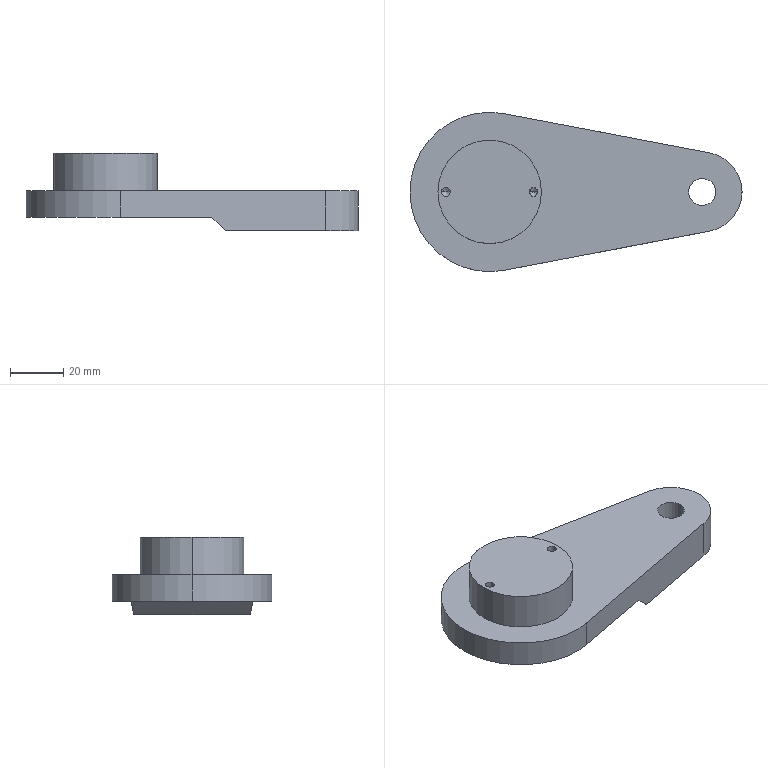Part | STEP file | Driven adjustment support (reverse) QY-1-27 | 1 solid | 22 faces | box 125 x 60 x 29 mm | volume 78443 mm3 | cylinder 11 | plane 7 | cone 4 | commonest cylinder face diameters 3.3 x4 10.2 x2 39 x2 60 x2 30 x1
STEP:
#1=CARTESIAN_POINT('',(0.,0.,0.));
#2=DIRECTION('',(0.,0.,1.));
#3=DIRECTION('',(1.,0.,0.));
#4=AXIS2_PLACEMENT_3D('',#1,#2,#3);
#5=CARTESIAN_POINT('',(-14.85,0.,10.));
#6=VERTEX_POINT('',#5);
#7=CARTESIAN_POINT('',(-14.85,0.,21.5));
#8=VERTEX_POINT('',#7);
#9=CARTESIAN_POINT('',(-14.85,0.,21.5));
#10=DIRECTION('',(0.,0.,1.));
#11=VECTOR('',#10,1.);
#12=LINE('',#9,#11);
#13=CARTESIAN_POINT('',(-16.5,0.,21.5));
#14=DIRECTION('',(0.,0.,1.));
#15=DIRECTION('',(1.,0.,0.));
#16=AXIS2_PLACEMENT_3D('',#13,#14,#15);
#17=CYLINDRICAL_SURFACE('',#16,1.65);
#18=CARTESIAN_POINT('',(6.283,0.));
#19=DIRECTION('',(0.,1.));
#20=VECTOR('',#19,1.);
#21=LINE('',#18,#20);
#22=(GEOMETRIC_REPRESENTATION_CONTEXT(2)PARAMETRIC_REPRESENTATION_CONTEXT()REPRESENTATION_CONTEXT('',''));
#23=DEFINITIONAL_REPRESENTATION('',(#21),#22);
#24=PCURVE('',#17,#23);
#25=CARTESIAN_POINT('',(-16.5,0.,21.5));
#26=DIRECTION('',(0.,0.,1.));
#27=DIRECTION('',(1.,0.,0.));
#28=AXIS2_PLACEMENT_3D('',#25,#26,#27);
#29=CYLINDRICAL_SURFACE('',#28,1.65);
#30=CARTESIAN_POINT('',(0.,0.));
#31=DIRECTION('',(0.,1.));
#32=VECTOR('',#31,1.);
#33=LINE('',#30,#32);
#34=(GEOMETRIC_REPRESENTATION_CONTEXT(2)PARAMETRIC_REPRESENTATION_CONTEXT()REPRESENTATION_CONTEXT('',''));
#35=DEFINITIONAL_REPRESENTATION('',(#33),#34);
#36=PCURVE('',#29,#35);
#37=SURFACE_CURVE('',#12,(#24,#36),.PCURVE_S1.);
#38=EDGE_CURVE('',#6,#8,#37,.T.);
#39=ORIENTED_EDGE('',*,*,#38,.T.);
#40=CARTESIAN_POINT('',(-18.15,0.,21.5));
#41=VERTEX_POINT('',#40);
#42=CARTESIAN_POINT('',(-16.5,0.,21.5));
#43=DIRECTION('',(0.,0.,1.));
#44=DIRECTION('',(1.,0.,0.));
#45=AXIS2_PLACEMENT_3D('',#42,#43,#44);
#46=CIRCLE('',#45,1.65);
#47=CARTESIAN_POINT('',(0.,0.));
#48=DIRECTION('',(1.,0.));
#49=VECTOR('',#48,1.);
#50=LINE('',#47,#49);
#51=(GEOMETRIC_REPRESENTATION_CONTEXT(2)PARAMETRIC_REPRESENTATION_CONTEXT()REPRESENTATION_CONTEXT('',''));
#52=DEFINITIONAL_REPRESENTATION('',(#50),#51);
#53=PCURVE('',#17,#52);
#54=CARTESIAN_POINT('',(0.,0.,21.5));
#55=DIRECTION('',(0.,0.,1.));
#56=DIRECTION('',(1.,0.,0.));
#57=AXIS2_PLACEMENT_3D('',#54,#55,#56);
#58=PLANE('',#57);
#59=CARTESIAN_POINT('',(-16.5,0.));
#60=DIRECTION('',(1.,0.));
#61=AXIS2_PLACEMENT_2D('',#59,#60);
#62=CIRCLE('',#61,1.65);
#63=(GEOMETRIC_REPRESENTATION_CONTEXT(2)PARAMETRIC_REPRESENTATION_CONTEXT()REPRESENTATION_CONTEXT('',''));
#64=DEFINITIONAL_REPRESENTATION('',(#62),#63);
#65=PCURVE('',#58,#64);
#66=SURFACE_CURVE('',#46,(#53,#65),.PCURVE_S1.);
#67=EDGE_CURVE('',#41,#8,#66,.T.);
#68=ORIENTED_EDGE('',*,*,#67,.F.);
#69=CARTESIAN_POINT('',(-18.15,0.,10.));
#70=VERTEX_POINT('',#69);
#71=CARTESIAN_POINT('',(-18.15,0.,21.5));
#72=DIRECTION('',(0.,0.,1.));
#73=VECTOR('',#72,1.);
#74=LINE('',#71,#73);
#75=CARTESIAN_POINT('',(3.142,0.));
#76=DIRECTION('',(0.,1.));
#77=VECTOR('',#76,1.);
#78=LINE('',#75,#77);
#79=(GEOMETRIC_REPRESENTATION_CONTEXT(2)PARAMETRIC_REPRESENTATION_CONTEXT()REPRESENTATION_CONTEXT('',''));
#80=DEFINITIONAL_REPRESENTATION('',(#78),#79);
#81=PCURVE('',#17,#80);
#82=CARTESIAN_POINT('',(3.142,0.));
#83=DIRECTION('',(0.,1.));
#84=VECTOR('',#83,1.);
#85=LINE('',#82,#84);
#86=(GEOMETRIC_REPRESENTATION_CONTEXT(2)PARAMETRIC_REPRESENTATION_CONTEXT()REPRESENTATION_CONTEXT('',''));
#87=DEFINITIONAL_REPRESENTATION('',(#85),#86);
#88=PCURVE('',#29,#87);
#89=SURFACE_CURVE('',#74,(#81,#88),.PCURVE_S1.);
#90=EDGE_CURVE('',#70,#41,#89,.T.);
#91=ORIENTED_EDGE('',*,*,#90,.F.);
#92=CARTESIAN_POINT('',(-16.5,0.,10.));
#93=DIRECTION('',(0.,0.,1.));
#94=DIRECTION('',(1.,0.,0.));
#95=AXIS2_PLACEMENT_3D('',#92,#93,#94);
#96=CIRCLE('',#95,1.65);
#97=CARTESIAN_POINT('',(0.,-11.5));
#98=DIRECTION('',(1.,0.));
#99=VECTOR('',#98,1.);
#100=LINE('',#97,#99);
#101=(GEOMETRIC_REPRESENTATION_CONTEXT(2)PARAMETRIC_REPRESENTATION_CONTEXT()REPRESENTATION_CONTEXT('',''));
#102=DEFINITIONAL_REPRESENTATION('',(#100),#101);
#103=PCURVE('',#17,#102);
#104=CARTESIAN_POINT('',(-16.5,0.,10.));
#105=DIRECTION('',(0.,0.,1.));
#106=DIRECTION('',(1.,0.,0.));
#107=AXIS2_PLACEMENT_3D('',#104,#105,#106);
#108=CONICAL_SURFACE('',#107,1.65,1.03);
#109=CARTESIAN_POINT('',(0.,0.));
#110=DIRECTION('',(1.,0.));
#111=VECTOR('',#110,1.);
#112=LINE('',#109,#111);
#113=(GEOMETRIC_REPRESENTATION_CONTEXT(2)PARAMETRIC_REPRESENTATION_CONTEXT()REPRESENTATION_CONTEXT('',''));
#114=DEFINITIONAL_REPRESENTATION('',(#112),#113);
#115=PCURVE('',#108,#114);
#116=SURFACE_CURVE('',#96,(#103,#115),.PCURVE_S1.);
#117=EDGE_CURVE('',#70,#6,#116,.T.);
#118=ORIENTED_EDGE('',*,*,#117,.T.);
#119=EDGE_LOOP('',(#39,#68,#91,#118));
#120=FACE_BOUND('',#119,.F.);
#121=ADVANCED_FACE('',(#120),#17,.F.);
#122=ORIENTED_EDGE('',*,*,#117,.F.);
#123=CARTESIAN_POINT('',(-16.5,0.,9.009));
#124=VERTEX_POINT('',#123);
#125=CARTESIAN_POINT('',(-18.15,0.,10.));
#126=DIRECTION('',(-0.8572,0.,0.515));
#127=VECTOR('',#126,1.);
#128=LINE('',#125,#127);
#129=CARTESIAN_POINT('',(3.142,0.));
#130=DIRECTION('',(0.,1.));
#131=VECTOR('',#130,1.);
#132=LINE('',#129,#131);
#133=(GEOMETRIC_REPRESENTATION_CONTEXT(2)PARAMETRIC_REPRESENTATION_CONTEXT()REPRESENTATION_CONTEXT('',''));
#134=DEFINITIONAL_REPRESENTATION('',(#132),#133);
#135=PCURVE('',#108,#134);
#136=CARTESIAN_POINT('',(-16.5,0.,10.));
#137=DIRECTION('',(0.,0.,1.));
#138=DIRECTION('',(1.,0.,0.));
#139=AXIS2_PLACEMENT_3D('',#136,#137,#138);
#140=CONICAL_SURFACE('',#139,1.65,1.03);
#141=CARTESIAN_POINT('',(3.142,0.));
#142=DIRECTION('',(0.,1.));
#143=VECTOR('',#142,1.);
#144=LINE('',#141,#143);
#145=(GEOMETRIC_REPRESENTATION_CONTEXT(2)PARAMETRIC_REPRESENTATION_CONTEXT()REPRESENTATION_CONTEXT('',''));
#146=DEFINITIONAL_REPRESENTATION('',(#144),#145);
#147=PCURVE('',#140,#146);
#148=SURFACE_CURVE('',#128,(#135,#147),.PCURVE_S1.);
#149=EDGE_CURVE('',#124,#70,#148,.T.);
#150=ORIENTED_EDGE('',*,*,#149,.F.);
#151=CARTESIAN_POINT('',(-14.85,0.,10.));
#152=DIRECTION('',(0.8572,0.,0.515));
#153=VECTOR('',#152,1.);
#154=LINE('',#151,#153);
#155=CARTESIAN_POINT('',(6.283,0.));
#156=DIRECTION('',(0.,1.));
#157=VECTOR('',#156,1.);
#158=LINE('',#155,#157);
#159=(GEOMETRIC_REPRESENTATION_CONTEXT(2)PARAMETRIC_REPRESENTATION_CONTEXT()REPRESENTATION_CONTEXT('',''));
#160=DEFINITIONAL_REPRESENTATION('',(#158),#159);
#161=PCURVE('',#108,#160);
#162=CARTESIAN_POINT('',(0.,0.));
#163=DIRECTION('',(0.,1.));
#164=VECTOR('',#163,1.);
#165=LINE('',#162,#164);
#166=(GEOMETRIC_REPRESENTATION_CONTEXT(2)PARAMETRIC_REPRESENTATION_CONTEXT()REPRESENTATION_CONTEXT('',''));
#167=DEFINITIONAL_REPRESENTATION('',(#165),#166);
#168=PCURVE('',#140,#167);
#169=SURFACE_CURVE('',#154,(#161,#168),.PCURVE_S1.);
#170=EDGE_CURVE('',#124,#6,#169,.T.);
#171=ORIENTED_EDGE('',*,*,#170,.T.);
#172=EDGE_LOOP('',(#122,#150,#171));
#173=FACE_BOUND('',#172,.F.);
#174=ADVANCED_FACE('',(#173),#108,.F.);
#175=CARTESIAN_POINT('',(18.15,0.,10.));
#176=VERTEX_POINT('',#175);
#177=CARTESIAN_POINT('',(18.15,0.,21.5));
#178=VERTEX_POINT('',#177);
#179=CARTESIAN_POINT('',(18.15,0.,21.5));
#180=DIRECTION('',(0.,0.,1.));
#181=VECTOR('',#180,1.);
#182=LINE('',#179,#181);
#183=CARTESIAN_POINT('',(16.5,0.,21.5));
#184=DIRECTION('',(0.,0.,1.));
#185=DIRECTION('',(1.,0.,0.));
#186=AXIS2_PLACEMENT_3D('',#183,#184,#185);
#187=CYLINDRICAL_SURFACE('',#186,1.65);
#188=CARTESIAN_POINT('',(6.283,0.));
#189=DIRECTION('',(0.,1.));
#190=VECTOR('',#189,1.);
#191=LINE('',#188,#190);
#192=(GEOMETRIC_REPRESENTATION_CONTEXT(2)PARAMETRIC_REPRESENTATION_CONTEXT()REPRESENTATION_CONTEXT('',''));
#193=DEFINITIONAL_REPRESENTATION('',(#191),#192);
#194=PCURVE('',#187,#193);
#195=CARTESIAN_POINT('',(16.5,0.,21.5));
#196=DIRECTION('',(0.,0.,1.));
#197=DIRECTION('',(1.,0.,0.));
#198=AXIS2_PLACEMENT_3D('',#195,#196,#197);
#199=CYLINDRICAL_SURFACE('',#198,1.65);
#200=CARTESIAN_POINT('',(0.,0.));
#201=DIRECTION('',(0.,1.));
#202=VECTOR('',#201,1.);
#203=LINE('',#200,#202);
#204=(GEOMETRIC_REPRESENTATION_CONTEXT(2)PARAMETRIC_REPRESENTATION_CONTEXT()REPRESENTATION_CONTEXT('',''));
#205=DEFINITIONAL_REPRESENTATION('',(#203),#204);
#206=PCURVE('',#199,#205);
#207=SURFACE_CURVE('',#182,(#194,#206),.PCURVE_S1.);
#208=EDGE_CURVE('',#176,#178,#207,.T.);
#209=ORIENTED_EDGE('',*,*,#208,.T.);
#210=CARTESIAN_POINT('',(14.85,0.,21.5));
#211=VERTEX_POINT('',#210);
#212=CARTESIAN_POINT('',(16.5,0.,21.5));
#213=DIRECTION('',(0.,0.,1.));
#214=DIRECTION('',(1.,0.,0.));
#215=AXIS2_PLACEMENT_3D('',#212,#213,#214);
#216=CIRCLE('',#215,1.65);
#217=CARTESIAN_POINT('',(0.,0.));
#218=DIRECTION('',(1.,0.));
#219=VECTOR('',#218,1.);
#220=LINE('',#217,#219);
#221=(GEOMETRIC_REPRESENTATION_CONTEXT(2)PARAMETRIC_REPRESENTATION_CONTEXT()REPRESENTATION_CONTEXT('',''));
#222=DEFINITIONAL_REPRESENTATION('',(#220),#221);
#223=PCURVE('',#187,#222);
#224=CARTESIAN_POINT('',(16.5,0.));
#225=DIRECTION('',(1.,0.));
#226=AXIS2_PLACEMENT_2D('',#224,#225);
#227=CIRCLE('',#226,1.65);
#228=(GEOMETRIC_REPRESENTATION_CONTEXT(2)PARAMETRIC_REPRESENTATION_CONTEXT()REPRESENTATION_CONTEXT('',''));
#229=DEFINITIONAL_REPRESENTATION('',(#227),#228);
#230=PCURVE('',#58,#229);
#231=SURFACE_CURVE('',#216,(#223,#230),.PCURVE_S1.);
#232=EDGE_CURVE('',#211,#178,#231,.T.);
#233=ORIENTED_EDGE('',*,*,#232,.F.);
#234=CARTESIAN_POINT('',(14.85,0.,10.));
#235=VERTEX_POINT('',#234);
#236=CARTESIAN_POINT('',(14.85,0.,21.5));
#237=DIRECTION('',(0.,0.,1.));
#238=VECTOR('',#237,1.);
#239=LINE('',#236,#238);
#240=CARTESIAN_POINT('',(3.142,0.));
#241=DIRECTION('',(0.,1.));
#242=VECTOR('',#241,1.);
#243=LINE('',#240,#242);
#244=(GEOMETRIC_REPRESENTATION_CONTEXT(2)PARAMETRIC_REPRESENTATION_CONTEXT()REPRESENTATION_CONTEXT('',''));
#245=DEFINITIONAL_REPRESENTATION('',(#243),#244);
#246=PCURVE('',#187,#245);
#247=CARTESIAN_POINT('',(3.142,0.));
#248=DIRECTION('',(0.,1.));
#249=VECTOR('',#248,1.);
#250=LINE('',#247,#249);
#251=(GEOMETRIC_REPRESENTATION_CONTEXT(2)PARAMETRIC_REPRESENTATION_CONTEXT()REPRESENTATION_CONTEXT('',''));
#252=DEFINITIONAL_REPRESENTATION('',(#250),#251);
#253=PCURVE('',#199,#252);
#254=SURFACE_CURVE('',#239,(#246,#253),.PCURVE_S1.);
#255=EDGE_CURVE('',#235,#211,#254,.T.);
#256=ORIENTED_EDGE('',*,*,#255,.F.);
#257=CARTESIAN_POINT('',(16.5,0.,10.));
#258=DIRECTION('',(0.,0.,1.));
#259=DIRECTION('',(1.,0.,0.));
#260=AXIS2_PLACEMENT_3D('',#257,#258,#259);
#261=CIRCLE('',#260,1.65);
#262=CARTESIAN_POINT('',(0.,-11.5));
#263=DIRECTION('',(1.,0.));
#264=VECTOR('',#263,1.);
#265=LINE('',#262,#264);
#266=(GEOMETRIC_REPRESENTATION_CONTEXT(2)PARAMETRIC_REPRESENTATION_CONTEXT()REPRESENTATION_CONTEXT('',''));
#267=DEFINITIONAL_REPRESENTATION('',(#265),#266);
#268=PCURVE('',#187,#267);
#269=CARTESIAN_POINT('',(16.5,0.,10.));
#270=DIRECTION('',(0.,0.,1.));
#271=DIRECTION('',(1.,0.,0.));
#272=AXIS2_PLACEMENT_3D('',#269,#270,#271);
#273=CONICAL_SURFACE('',#272,1.65,1.03);
#274=CARTESIAN_POINT('',(0.,0.));
#275=DIRECTION('',(1.,0.));
#276=VECTOR('',#275,1.);
#277=LINE('',#274,#276);
#278=(GEOMETRIC_REPRESENTATION_CONTEXT(2)PARAMETRIC_REPRESENTATION_CONTEXT()REPRESENTATION_CONTEXT('',''));
#279=DEFINITIONAL_REPRESENTATION('',(#277),#278);
#280=PCURVE('',#273,#279);
#281=SURFACE_CURVE('',#261,(#268,#280),.PCURVE_S1.);
#282=EDGE_CURVE('',#235,#176,#281,.T.);
#283=ORIENTED_EDGE('',*,*,#282,.T.);
#284=EDGE_LOOP('',(#209,#233,#256,#283));
#285=FACE_BOUND('',#284,.F.);
#286=ADVANCED_FACE('',(#285),#187,.F.);
#287=ORIENTED_EDGE('',*,*,#282,.F.);
#288=CARTESIAN_POINT('',(16.5,0.,9.009));
#289=VERTEX_POINT('',#288);
#290=CARTESIAN_POINT('',(14.85,0.,10.));
#291=DIRECTION('',(-0.8572,0.,0.515));
#292=VECTOR('',#291,1.);
#293=LINE('',#290,#292);
#294=CARTESIAN_POINT('',(3.142,0.));
#295=DIRECTION('',(0.,1.));
#296=VECTOR('',#295,1.);
#297=LINE('',#294,#296);
#298=(GEOMETRIC_REPRESENTATION_CONTEXT(2)PARAMETRIC_REPRESENTATION_CONTEXT()REPRESENTATION_CONTEXT('',''));
#299=DEFINITIONAL_REPRESENTATION('',(#297),#298);
#300=PCURVE('',#273,#299);
#301=CARTESIAN_POINT('',(16.5,0.,10.));
#302=DIRECTION('',(0.,0.,1.));
#303=DIRECTION('',(1.,0.,0.));
#304=AXIS2_PLACEMENT_3D('',#301,#302,#303);
#305=CONICAL_SURFACE('',#304,1.65,1.03);
#306=CARTESIAN_POINT('',(3.142,0.));
#307=DIRECTION('',(0.,1.));
#308=VECTOR('',#307,1.);
#309=LINE('',#306,#308);
#310=(GEOMETRIC_REPRESENTATION_CONTEXT(2)PARAMETRIC_REPRESENTATION_CONTEXT()REPRESENTATION_CONTEXT('',''));
#311=DEFINITIONAL_REPRESENTATION('',(#309),#310);
#312=PCURVE('',#305,#311);
#313=SURFACE_CURVE('',#293,(#300,#312),.PCURVE_S1.);
#314=EDGE_CURVE('',#289,#235,#313,.T.);
#315=ORIENTED_EDGE('',*,*,#314,.F.);
#316=CARTESIAN_POINT('',(18.15,0.,10.));
#317=DIRECTION('',(0.8572,0.,0.515));
#318=VECTOR('',#317,1.);
#319=LINE('',#316,#318);
#320=CARTESIAN_POINT('',(6.283,0.));
#321=DIRECTION('',(0.,1.));
#322=VECTOR('',#321,1.);
#323=LINE('',#320,#322);
#324=(GEOMETRIC_REPRESENTATION_CONTEXT(2)PARAMETRIC_REPRESENTATION_CONTEXT()REPRESENTATION_CONTEXT('',''));
#325=DEFINITIONAL_REPRESENTATION('',(#323),#324);
#326=PCURVE('',#273,#325);
#327=CARTESIAN_POINT('',(0.,0.));
#328=DIRECTION('',(0.,1.));
#329=VECTOR('',#328,1.);
#330=LINE('',#327,#329);
#331=(GEOMETRIC_REPRESENTATION_CONTEXT(2)PARAMETRIC_REPRESENTATION_CONTEXT()REPRESENTATION_CONTEXT('',''));
#332=DEFINITIONAL_REPRESENTATION('',(#330),#331);
#333=PCURVE('',#305,#332);
#334=SURFACE_CURVE('',#319,(#326,#333),.PCURVE_S1.);
#335=EDGE_CURVE('',#289,#176,#334,.T.);
#336=ORIENTED_EDGE('',*,*,#335,.T.);
#337=EDGE_LOOP('',(#287,#315,#336));
#338=FACE_BOUND('',#337,.F.);
#339=ADVANCED_FACE('',(#338),#273,.F.);
#340=CARTESIAN_POINT('',(19.5,0.,21.5));
#341=VERTEX_POINT('',#340);
#342=CARTESIAN_POINT('',(-19.5,0.,21.5));
#343=VERTEX_POINT('',#342);
#344=CARTESIAN_POINT('',(0.,0.,21.5));
#345=DIRECTION('',(0.,0.,1.));
#346=DIRECTION('',(1.,0.,0.));
#347=AXIS2_PLACEMENT_3D('',#344,#345,#346);
#348=CIRCLE('',#347,19.5);
#349=CARTESIAN_POINT('',(0.,0.,21.5));
#350=DIRECTION('',(0.,0.,-1.));
#351=DIRECTION('',(-1.,0.,0.));
#352=AXIS2_PLACEMENT_3D('',#349,#350,#351);
#353=CYLINDRICAL_SURFACE('',#352,19.5);
#354=CARTESIAN_POINT('',(3.142,0.));
#355=DIRECTION('',(-1.,0.));
#356=VECTOR('',#355,1.);
#357=LINE('',#354,#356);
#358=(GEOMETRIC_REPRESENTATION_CONTEXT(2)PARAMETRIC_REPRESENTATION_CONTEXT()REPRESENTATION_CONTEXT('',''));
#359=DEFINITIONAL_REPRESENTATION('',(#357),#358);
#360=PCURVE('',#353,#359);
#361=CARTESIAN_POINT('',(0.,0.));
#362=DIRECTION('',(1.,0.));
#363=AXIS2_PLACEMENT_2D('',#361,#362);
#364=CIRCLE('',#363,19.5);
#365=(GEOMETRIC_REPRESENTATION_CONTEXT(2)PARAMETRIC_REPRESENTATION_CONTEXT()REPRESENTATION_CONTEXT('',''));
#366=DEFINITIONAL_REPRESENTATION('',(#364),#365);
#367=PCURVE('',#58,#366);
#368=SURFACE_CURVE('',#348,(#360,#367),.PCURVE_S1.);
#369=EDGE_CURVE('',#341,#343,#368,.T.);
#370=ORIENTED_EDGE('',*,*,#369,.F.);
#371=CARTESIAN_POINT('',(19.5,0.,7.5));
#372=VERTEX_POINT('',#371);
#373=CARTESIAN_POINT('',(19.5,0.,21.5));
#374=DIRECTION('',(0.,0.,-1.));
#375=VECTOR('',#374,1.);
#376=LINE('',#373,#375);
#377=CARTESIAN_POINT('',(3.142,0.));
#378=DIRECTION('',(0.,1.));
#379=VECTOR('',#378,1.);
#380=LINE('',#377,#379);
#381=(GEOMETRIC_REPRESENTATION_CONTEXT(2)PARAMETRIC_REPRESENTATION_CONTEXT()REPRESENTATION_CONTEXT('',''));
#382=DEFINITIONAL_REPRESENTATION('',(#380),#381);
#383=PCURVE('',#353,#382);
#384=CARTESIAN_POINT('',(0.,0.,21.5));
#385=DIRECTION('',(0.,0.,-1.));
#386=DIRECTION('',(-1.,0.,0.));
#387=AXIS2_PLACEMENT_3D('',#384,#385,#386);
#388=CYLINDRICAL_SURFACE('',#387,19.5);
#389=CARTESIAN_POINT('',(3.142,0.));
#390=DIRECTION('',(0.,1.));
#391=VECTOR('',#390,1.);
#392=LINE('',#389,#391);
#393=(GEOMETRIC_REPRESENTATION_CONTEXT(2)PARAMETRIC_REPRESENTATION_CONTEXT()REPRESENTATION_CONTEXT('',''));
#394=DEFINITIONAL_REPRESENTATION('',(#392),#393);
#395=PCURVE('',#388,#394);
#396=SURFACE_CURVE('',#376,(#383,#395),.PCURVE_S1.);
#397=EDGE_CURVE('',#341,#372,#396,.T.);
#398=ORIENTED_EDGE('',*,*,#397,.T.);
#399=CARTESIAN_POINT('',(-19.5,0.,7.5));
#400=VERTEX_POINT('',#399);
#401=CARTESIAN_POINT('',(0.,0.,7.5));
#402=DIRECTION('',(0.,0.,1.));
#403=DIRECTION('',(1.,0.,0.));
#404=AXIS2_PLACEMENT_3D('',#401,#402,#403);
#405=CIRCLE('',#404,19.5);
#406=CARTESIAN_POINT('',(3.142,14.));
#407=DIRECTION('',(-1.,0.));
#408=VECTOR('',#407,1.);
#409=LINE('',#406,#408);
#410=(GEOMETRIC_REPRESENTATION_CONTEXT(2)PARAMETRIC_REPRESENTATION_CONTEXT()REPRESENTATION_CONTEXT('',''));
#411=DEFINITIONAL_REPRESENTATION('',(#409),#410);
#412=PCURVE('',#353,#411);
#413=CARTESIAN_POINT('',(0.,0.,7.5));
#414=DIRECTION('',(0.,0.,1.));
#415=DIRECTION('',(1.,0.,0.));
#416=AXIS2_PLACEMENT_3D('',#413,#414,#415);
#417=PLANE('',#416);
#418=CARTESIAN_POINT('',(0.,0.));
#419=DIRECTION('',(1.,0.));
#420=AXIS2_PLACEMENT_2D('',#418,#419);
#421=CIRCLE('',#420,19.5);
#422=(GEOMETRIC_REPRESENTATION_CONTEXT(2)PARAMETRIC_REPRESENTATION_CONTEXT()REPRESENTATION_CONTEXT('',''));
#423=DEFINITIONAL_REPRESENTATION('',(#421),#422);
#424=PCURVE('',#417,#423);
#425=SURFACE_CURVE('',#405,(#412,#424),.PCURVE_S1.);
#426=EDGE_CURVE('',#372,#400,#425,.T.);
#427=ORIENTED_EDGE('',*,*,#426,.T.);
#428=CARTESIAN_POINT('',(-19.5,0.,21.5));
#429=DIRECTION('',(0.,0.,-1.));
#430=VECTOR('',#429,1.);
#431=LINE('',#428,#430);
#432=CARTESIAN_POINT('',(0.,0.));
#433=DIRECTION('',(0.,1.));
#434=VECTOR('',#433,1.);
#435=LINE('',#432,#434);
#436=(GEOMETRIC_REPRESENTATION_CONTEXT(2)PARAMETRIC_REPRESENTATION_CONTEXT()REPRESENTATION_CONTEXT('',''));
#437=DEFINITIONAL_REPRESENTATION('',(#435),#436);
#438=PCURVE('',#353,#437);
#439=CARTESIAN_POINT('',(6.283,0.));
#440=DIRECTION('',(0.,1.));
#441=VECTOR('',#440,1.);
#442=LINE('',#439,#441);
#443=(GEOMETRIC_REPRESENTATION_CONTEXT(2)PARAMETRIC_REPRESENTATION_CONTEXT()REPRESENTATION_CONTEXT('',''));
#444=DEFINITIONAL_REPRESENTATION('',(#442),#443);
#445=PCURVE('',#388,#444);
#446=SURFACE_CURVE('',#431,(#438,#445),.PCURVE_S1.);
#447=EDGE_CURVE('',#343,#400,#446,.T.);
#448=ORIENTED_EDGE('',*,*,#447,.F.);
#449=EDGE_LOOP('',(#370,#398,#427,#448));
#450=FACE_BOUND('',#449,.T.);
#451=ADVANCED_FACE('',(#450),#353,.T.);
#452=CARTESIAN_POINT('',(74.9,0.,7.5));
#453=VERTEX_POINT('',#452);
#454=CARTESIAN_POINT('',(74.9,0.,-7.5));
#455=VERTEX_POINT('',#454);
#456=CARTESIAN_POINT('',(74.9,0.,-7.5));
#457=DIRECTION('',(0.,0.,-1.));
#458=VECTOR('',#457,1.);
#459=LINE('',#456,#458);
#460=CARTESIAN_POINT('',(80.,0.,-7.5));
#461=DIRECTION('',(0.,0.,-1.));
#462=DIRECTION('',(-1.,0.,0.));
#463=AXIS2_PLACEMENT_3D('',#460,#461,#462);
#464=CYLINDRICAL_SURFACE('',#463,5.1);
#465=CARTESIAN_POINT('',(6.283,0.));
#466=DIRECTION('',(0.,1.));
#467=VECTOR('',#466,1.);
#468=LINE('',#465,#467);
#469=(GEOMETRIC_REPRESENTATION_CONTEXT(2)PARAMETRIC_REPRESENTATION_CONTEXT()REPRESENTATION_CONTEXT('',''));
#470=DEFINITIONAL_REPRESENTATION('',(#468),#469);
#471=PCURVE('',#464,#470);
#472=CARTESIAN_POINT('',(80.,0.,-7.5));
#473=DIRECTION('',(0.,0.,-1.));
#474=DIRECTION('',(-1.,0.,0.));
#475=AXIS2_PLACEMENT_3D('',#472,#473,#474);
#476=CYLINDRICAL_SURFACE('',#475,5.1);
#477=CARTESIAN_POINT('',(0.,0.));
#478=DIRECTION('',(0.,1.));
#479=VECTOR('',#478,1.);
#480=LINE('',#477,#479);
#481=(GEOMETRIC_REPRESENTATION_CONTEXT(2)PARAMETRIC_REPRESENTATION_CONTEXT()REPRESENTATION_CONTEXT('',''));
#482=DEFINITIONAL_REPRESENTATION('',(#480),#481);
#483=PCURVE('',#476,#482);
#484=SURFACE_CURVE('',#459,(#471,#483),.PCURVE_S1.);
#485=EDGE_CURVE('',#453,#455,#484,.T.);
#486=ORIENTED_EDGE('',*,*,#485,.T.);
#487=CARTESIAN_POINT('',(85.1,0.,-7.5));
#488=VERTEX_POINT('',#487);
#489=CARTESIAN_POINT('',(80.,0.,-7.5));
#490=DIRECTION('',(0.,0.,-1.));
#491=DIRECTION('',(-1.,0.,0.));
#492=AXIS2_PLACEMENT_3D('',#489,#490,#491);
#493=CIRCLE('',#492,5.1);
#494=CARTESIAN_POINT('',(0.,0.));
#495=DIRECTION('',(1.,0.));
#496=VECTOR('',#495,1.);
#497=LINE('',#494,#496);
#498=(GEOMETRIC_REPRESENTATION_CONTEXT(2)PARAMETRIC_REPRESENTATION_CONTEXT()REPRESENTATION_CONTEXT('',''));
#499=DEFINITIONAL_REPRESENTATION('',(#497),#498);
#500=PCURVE('',#464,#499);
#501=CARTESIAN_POINT('',(0.,0.,-7.5));
#502=DIRECTION('',(0.,0.,1.));
#503=DIRECTION('',(1.,0.,0.));
#504=AXIS2_PLACEMENT_3D('',#501,#502,#503);
#505=PLANE('',#504);
#506=CARTESIAN_POINT('',(74.9,0.));
#507=CARTESIAN_POINT('',(74.9,8.833));
#508=CARTESIAN_POINT('',(82.55,4.417));
#509=CARTESIAN_POINT('',(90.2,0.));
#510=CARTESIAN_POINT('',(82.55,-4.417));
#511=CARTESIAN_POINT('',(74.9,-8.833));
#512=CARTESIAN_POINT('',(74.9,0.));
#513=(BOUNDED_CURVE()B_SPLINE_CURVE(2,(#506,#507,#508,#509,#510,#511,#512),.UNSPECIFIED.,.T.,.F.)B_SPLINE_CURVE_WITH_KNOTS((1,2,2,2,2,1),(-2.094,0.,2.094,4.189,6.283,8.378),.UNSPECIFIED.)CURVE()GEOMETRIC_REPRESENTATION_ITEM()RATIONAL_B_SPLINE_CURVE((1.,0.5,1.,0.5,1.,0.5,1.))REPRESENTATION_ITEM(''));
#514=(GEOMETRIC_REPRESENTATION_CONTEXT(2)PARAMETRIC_REPRESENTATION_CONTEXT()REPRESENTATION_CONTEXT('',''));
#515=DEFINITIONAL_REPRESENTATION('',(#513),#514);
#516=PCURVE('',#505,#515);
#517=SURFACE_CURVE('',#493,(#500,#516),.PCURVE_S1.);
#518=EDGE_CURVE('',#488,#455,#517,.T.);
#519=ORIENTED_EDGE('',*,*,#518,.F.);
#520=CARTESIAN_POINT('',(85.1,0.,7.5));
#521=VERTEX_POINT('',#520);
#522=CARTESIAN_POINT('',(85.1,0.,-7.5));
#523=DIRECTION('',(0.,0.,-1.));
#524=VECTOR('',#523,1.);
#525=LINE('',#522,#524);
#526=CARTESIAN_POINT('',(3.142,0.));
#527=DIRECTION('',(0.,1.));
#528=VECTOR('',#527,1.);
#529=LINE('',#526,#528);
#530=(GEOMETRIC_REPRESENTATION_CONTEXT(2)PARAMETRIC_REPRESENTATION_CONTEXT()REPRESENTATION_CONTEXT('',''));
#531=DEFINITIONAL_REPRESENTATION('',(#529),#530);
#532=PCURVE('',#464,#531);
#533=CARTESIAN_POINT('',(3.142,0.));
#534=DIRECTION('',(0.,1.));
#535=VECTOR('',#534,1.);
#536=LINE('',#533,#535);
#537=(GEOMETRIC_REPRESENTATION_CONTEXT(2)PARAMETRIC_REPRESENTATION_CONTEXT()REPRESENTATION_CONTEXT('',''));
#538=DEFINITIONAL_REPRESENTATION('',(#536),#537);
#539=PCURVE('',#476,#538);
#540=SURFACE_CURVE('',#525,(#532,#539),.PCURVE_S1.);
#541=EDGE_CURVE('',#521,#488,#540,.T.);
#542=ORIENTED_EDGE('',*,*,#541,.F.);
#543=CARTESIAN_POINT('',(80.,0.,7.5));
#544=DIRECTION('',(0.,0.,1.));
#545=DIRECTION('',(1.,0.,0.));
#546=AXIS2_PLACEMENT_3D('',#543,#544,#545);
#547=CIRCLE('',#546,5.1);
#548=CARTESIAN_POINT('',(9.425,-15.));
#549=DIRECTION('',(-1.,0.));
#550=VECTOR('',#549,1.);
#551=LINE('',#548,#550);
#552=(GEOMETRIC_REPRESENTATION_CONTEXT(2)PARAMETRIC_REPRESENTATION_CONTEXT()REPRESENTATION_CONTEXT('',''));
#553=DEFINITIONAL_REPRESENTATION('',(#551),#552);
#554=PCURVE('',#464,#553);
#555=CARTESIAN_POINT('',(80.,0.));
#556=DIRECTION('',(1.,0.));
#557=AXIS2_PLACEMENT_2D('',#555,#556);
#558=CIRCLE('',#557,5.1);
#559=(GEOMETRIC_REPRESENTATION_CONTEXT(2)PARAMETRIC_REPRESENTATION_CONTEXT()REPRESENTATION_CONTEXT('',''));
#560=DEFINITIONAL_REPRESENTATION('',(#558),#559);
#561=PCURVE('',#417,#560);
#562=SURFACE_CURVE('',#547,(#554,#561),.PCURVE_S1.);
#563=EDGE_CURVE('',#453,#521,#562,.T.);
#564=ORIENTED_EDGE('',*,*,#563,.F.);
#565=EDGE_LOOP('',(#486,#519,#542,#564));
#566=FACE_BOUND('',#565,.F.);
#567=ADVANCED_FACE('',(#566),#464,.F.);
#568=CARTESIAN_POINT('',(-30.,0.,7.5));
#569=VERTEX_POINT('',#568);
#570=CARTESIAN_POINT('',(5.625,-29.468,7.5));
#571=VERTEX_POINT('',#570);
#572=CARTESIAN_POINT('',(0.,0.,7.5));
#573=DIRECTION('',(0.,0.,1.));
#574=DIRECTION('',(1.,0.,0.));
#575=AXIS2_PLACEMENT_3D('',#572,#573,#574);
#576=CIRCLE('',#575,30.);
#577=CARTESIAN_POINT('',(0.,0.,7.5));
#578=DIRECTION('',(0.,0.,-1.));
#579=DIRECTION('',(-1.,0.,0.));
#580=AXIS2_PLACEMENT_3D('',#577,#578,#579);
#581=CYLINDRICAL_SURFACE('',#580,30.);
#582=CARTESIAN_POINT('',(9.425,0.));
#583=DIRECTION('',(-1.,0.));
#584=VECTOR('',#583,1.);
#585=LINE('',#582,#584);
#586=(GEOMETRIC_REPRESENTATION_CONTEXT(2)PARAMETRIC_REPRESENTATION_CONTEXT()REPRESENTATION_CONTEXT('',''));
#587=DEFINITIONAL_REPRESENTATION('',(#585),#586);
#588=PCURVE('',#581,#587);
#589=CARTESIAN_POINT('',(0.,0.));
#590=DIRECTION('',(1.,0.));
#591=AXIS2_PLACEMENT_2D('',#589,#590);
#592=CIRCLE('',#591,30.);
#593=(GEOMETRIC_REPRESENTATION_CONTEXT(2)PARAMETRIC_REPRESENTATION_CONTEXT()REPRESENTATION_CONTEXT('',''));
#594=DEFINITIONAL_REPRESENTATION('',(#592),#593);
#595=PCURVE('',#417,#594);
#596=SURFACE_CURVE('',#576,(#588,#595),.PCURVE_S1.);
#597=EDGE_CURVE('',#569,#571,#596,.T.);
#598=ORIENTED_EDGE('',*,*,#597,.F.);
#599=CARTESIAN_POINT('',(-30.,0.,-2.5));
#600=VERTEX_POINT('',#599);
#601=CARTESIAN_POINT('',(-30.,0.,7.5));
#602=DIRECTION('',(0.,0.,-1.));
#603=VECTOR('',#602,1.);
#604=LINE('',#601,#603);
#605=CARTESIAN_POINT('',(6.283,0.));
#606=DIRECTION('',(0.,1.));
#607=VECTOR('',#606,1.);
#608=LINE('',#605,#607);
#609=(GEOMETRIC_REPRESENTATION_CONTEXT(2)PARAMETRIC_REPRESENTATION_CONTEXT()REPRESENTATION_CONTEXT('',''));
#610=DEFINITIONAL_REPRESENTATION('',(#608),#609);
#611=PCURVE('',#581,#610);
#612=CARTESIAN_POINT('',(0.,0.,7.5));
#613=DIRECTION('',(0.,0.,-1.));
#614=DIRECTION('',(-1.,0.,0.));
#615=AXIS2_PLACEMENT_3D('',#612,#613,#614);
#616=CYLINDRICAL_SURFACE('',#615,30.);
#617=CARTESIAN_POINT('',(0.,0.));
#618=DIRECTION('',(0.,1.));
#619=VECTOR('',#618,1.);
#620=LINE('',#617,#619);
#621=(GEOMETRIC_REPRESENTATION_CONTEXT(2)PARAMETRIC_REPRESENTATION_CONTEXT()REPRESENTATION_CONTEXT('',''));
#622=DEFINITIONAL_REPRESENTATION('',(#620),#621);
#623=PCURVE('',#616,#622);
#624=SURFACE_CURVE('',#604,(#611,#623),.PCURVE_S1.);
#625=EDGE_CURVE('',#569,#600,#624,.T.);
#626=ORIENTED_EDGE('',*,*,#625,.T.);
#627=CARTESIAN_POINT('',(5.625,-29.468,-2.5));
#628=VERTEX_POINT('',#627);
#629=CARTESIAN_POINT('',(0.,0.,-2.5));
#630=DIRECTION('',(0.,0.,1.));
#631=DIRECTION('',(1.,0.,0.));
#632=AXIS2_PLACEMENT_3D('',#629,#630,#631);
#633=CIRCLE('',#632,30.);
#634=CARTESIAN_POINT('',(9.425,10.));
#635=DIRECTION('',(-1.,0.));
#636=VECTOR('',#635,1.);
#637=LINE('',#634,#636);
#638=(GEOMETRIC_REPRESENTATION_CONTEXT(2)PARAMETRIC_REPRESENTATION_CONTEXT()REPRESENTATION_CONTEXT('',''));
#639=DEFINITIONAL_REPRESENTATION('',(#637),#638);
#640=PCURVE('',#581,#639);
#641=CARTESIAN_POINT('',(-30.,-50.,-2.5));
#642=DIRECTION('',(0.,0.,1.));
#643=DIRECTION('',(1.,0.,0.));
#644=AXIS2_PLACEMENT_3D('',#641,#642,#643);
#645=PLANE('',#644);
#646=CARTESIAN_POINT('',(30.,50.));
#647=DIRECTION('',(1.,0.));
#648=AXIS2_PLACEMENT_2D('',#646,#647);
#649=CIRCLE('',#648,30.);
#650=(GEOMETRIC_REPRESENTATION_CONTEXT(2)PARAMETRIC_REPRESENTATION_CONTEXT()REPRESENTATION_CONTEXT('',''));
#651=DEFINITIONAL_REPRESENTATION('',(#649),#650);
#652=PCURVE('',#645,#651);
#653=SURFACE_CURVE('',#633,(#640,#652),.PCURVE_S1.);
#654=EDGE_CURVE('',#600,#628,#653,.T.);
#655=ORIENTED_EDGE('',*,*,#654,.T.);
#656=CARTESIAN_POINT('',(5.625,-29.468,7.5));
#657=DIRECTION('',(0.,0.,-1.));
#658=VECTOR('',#657,1.);
#659=LINE('',#656,#658);
#660=CARTESIAN_POINT('',(4.524,0.));
#661=DIRECTION('',(0.,1.));
#662=VECTOR('',#661,1.);
#663=LINE('',#660,#662);
#664=(GEOMETRIC_REPRESENTATION_CONTEXT(2)PARAMETRIC_REPRESENTATION_CONTEXT()REPRESENTATION_CONTEXT('',''));
#665=DEFINITIONAL_REPRESENTATION('',(#663),#664);
#666=PCURVE('',#581,#665);
#667=CARTESIAN_POINT('',(5.625,-29.468,7.5));
#668=DIRECTION('',(-0.1875,0.9823,0.));
#669=DIRECTION('',(-0.9823,-0.1875,0.));
#670=AXIS2_PLACEMENT_3D('',#667,#668,#669);
#671=PLANE('',#670);
#672=CARTESIAN_POINT('',(0.,0.));
#673=DIRECTION('',(0.,-1.));
#674=VECTOR('',#673,1.);
#675=LINE('',#672,#674);
#676=(GEOMETRIC_REPRESENTATION_CONTEXT(2)PARAMETRIC_REPRESENTATION_CONTEXT()REPRESENTATION_CONTEXT('',''));
#677=DEFINITIONAL_REPRESENTATION('',(#675),#676);
#678=PCURVE('',#671,#677);
#679=SURFACE_CURVE('',#659,(#666,#678),.PCURVE_S1.);
#680=EDGE_CURVE('',#571,#628,#679,.T.);
#681=ORIENTED_EDGE('',*,*,#680,.F.);
#682=EDGE_LOOP('',(#598,#626,#655,#681));
#683=FACE_BOUND('',#682,.T.);
#684=ADVANCED_FACE('',(#683),#581,.T.);
#685=ORIENTED_EDGE('',*,*,#625,.F.);
#686=CARTESIAN_POINT('',(5.625,29.468,7.5));
#687=VERTEX_POINT('',#686);
#688=CARTESIAN_POINT('',(0.,0.,7.5));
#689=DIRECTION('',(0.,0.,1.));
#690=DIRECTION('',(1.,0.,0.));
#691=AXIS2_PLACEMENT_3D('',#688,#689,#690);
#692=CIRCLE('',#691,30.);
#693=CARTESIAN_POINT('',(3.142,0.));
#694=DIRECTION('',(-1.,0.));
#695=VECTOR('',#694,1.);
#696=LINE('',#693,#695);
#697=(GEOMETRIC_REPRESENTATION_CONTEXT(2)PARAMETRIC_REPRESENTATION_CONTEXT()REPRESENTATION_CONTEXT('',''));
#698=DEFINITIONAL_REPRESENTATION('',(#696),#697);
#699=PCURVE('',#616,#698);
#700=CARTESIAN_POINT('',(0.,0.));
#701=DIRECTION('',(1.,0.));
#702=AXIS2_PLACEMENT_2D('',#700,#701);
#703=CIRCLE('',#702,30.);
#704=(GEOMETRIC_REPRESENTATION_CONTEXT(2)PARAMETRIC_REPRESENTATION_CONTEXT()REPRESENTATION_CONTEXT('',''));
#705=DEFINITIONAL_REPRESENTATION('',(#703),#704);
#706=PCURVE('',#417,#705);
#707=SURFACE_CURVE('',#692,(#699,#706),.PCURVE_S1.);
#708=EDGE_CURVE('',#687,#569,#707,.T.);
#709=ORIENTED_EDGE('',*,*,#708,.F.);
#710=CARTESIAN_POINT('',(5.625,29.468,-2.5));
#711=VERTEX_POINT('',#710);
#712=CARTESIAN_POINT('',(5.625,29.468,7.5));
#713=DIRECTION('',(0.,0.,-1.));
#714=VECTOR('',#713,1.);
#715=LINE('',#712,#714);
#716=CARTESIAN_POINT('',(1.759,0.));
#717=DIRECTION('',(0.,1.));
#718=VECTOR('',#717,1.);
#719=LINE('',#716,#718);
#720=(GEOMETRIC_REPRESENTATION_CONTEXT(2)PARAMETRIC_REPRESENTATION_CONTEXT()REPRESENTATION_CONTEXT('',''));
#721=DEFINITIONAL_REPRESENTATION('',(#719),#720);
#722=PCURVE('',#616,#721);
#723=CARTESIAN_POINT('',(5.625,29.468,7.5));
#724=DIRECTION('',(-0.1875,-0.9823,0.));
#725=DIRECTION('',(0.9823,-0.1875,0.));
#726=AXIS2_PLACEMENT_3D('',#723,#724,#725);
#727=PLANE('',#726);
#728=CARTESIAN_POINT('',(0.,0.));
#729=DIRECTION('',(0.,-1.));
#730=VECTOR('',#729,1.);
#731=LINE('',#728,#730);
#732=(GEOMETRIC_REPRESENTATION_CONTEXT(2)PARAMETRIC_REPRESENTATION_CONTEXT()REPRESENTATION_CONTEXT('',''));
#733=DEFINITIONAL_REPRESENTATION('',(#731),#732);
#734=PCURVE('',#727,#733);
#735=SURFACE_CURVE('',#715,(#722,#734),.PCURVE_S1.);
#736=EDGE_CURVE('',#687,#711,#735,.T.);
#737=ORIENTED_EDGE('',*,*,#736,.T.);
#738=CARTESIAN_POINT('',(0.,0.,-2.5));
#739=DIRECTION('',(0.,0.,1.));
#740=DIRECTION('',(1.,0.,0.));
#741=AXIS2_PLACEMENT_3D('',#738,#739,#740);
#742=CIRCLE('',#741,30.);
#743=CARTESIAN_POINT('',(3.142,10.));
#744=DIRECTION('',(-1.,0.));
#745=VECTOR('',#744,1.);
#746=LINE('',#743,#745);
#747=(GEOMETRIC_REPRESENTATION_CONTEXT(2)PARAMETRIC_REPRESENTATION_CONTEXT()REPRESENTATION_CONTEXT('',''));
#748=DEFINITIONAL_REPRESENTATION('',(#746),#747);
#749=PCURVE('',#616,#748);
#750=CARTESIAN_POINT('',(30.,50.));
#751=DIRECTION('',(1.,0.));
#752=AXIS2_PLACEMENT_2D('',#750,#751);
#753=CIRCLE('',#752,30.);
#754=(GEOMETRIC_REPRESENTATION_CONTEXT(2)PARAMETRIC_REPRESENTATION_CONTEXT()REPRESENTATION_CONTEXT('',''));
#755=DEFINITIONAL_REPRESENTATION('',(#753),#754);
#756=PCURVE('',#645,#755);
#757=SURFACE_CURVE('',#742,(#749,#756),.PCURVE_S1.);
#758=EDGE_CURVE('',#711,#600,#757,.T.);
#759=ORIENTED_EDGE('',*,*,#758,.T.);
#760=EDGE_LOOP('',(#685,#709,#737,#759));
#761=FACE_BOUND('',#760,.T.);
#762=ADVANCED_FACE('',(#761),#616,.T.);
#763=CARTESIAN_POINT('',(40.,-22.906,-2.5));
#764=VERTEX_POINT('',#763);
#765=CARTESIAN_POINT('',(5.625,-29.468,-2.5));
#766=DIRECTION('',(0.9823,0.1875,0.));
#767=VECTOR('',#766,1.);
#768=LINE('',#765,#767);
#769=CARTESIAN_POINT('',(0.,-10.));
#770=DIRECTION('',(-1.,0.));
#771=VECTOR('',#770,1.);
#772=LINE('',#769,#771);
#773=(GEOMETRIC_REPRESENTATION_CONTEXT(2)PARAMETRIC_REPRESENTATION_CONTEXT()REPRESENTATION_CONTEXT('',''));
#774=DEFINITIONAL_REPRESENTATION('',(#772),#773);
#775=PCURVE('',#671,#774);
#776=CARTESIAN_POINT('',(35.625,20.532));
#777=DIRECTION('',(0.9823,0.1875));
#778=VECTOR('',#777,1.);
#779=LINE('',#776,#778);
#780=(GEOMETRIC_REPRESENTATION_CONTEXT(2)PARAMETRIC_REPRESENTATION_CONTEXT()REPRESENTATION_CONTEXT('',''));
#781=DEFINITIONAL_REPRESENTATION('',(#779),#780);
#782=PCURVE('',#645,#781);
#783=SURFACE_CURVE('',#768,(#775,#782),.PCURVE_S1.);
#784=EDGE_CURVE('',#628,#764,#783,.T.);
#785=ORIENTED_EDGE('',*,*,#784,.T.);
#786=CARTESIAN_POINT('',(45.,-21.952,-7.5));
#787=VERTEX_POINT('',#786);
#788=CARTESIAN_POINT('',(17.594,-27.183,19.906));
#789=DIRECTION('',(0.7008,0.1338,-0.7008));
#790=VECTOR('',#789,1.);
#791=LINE('',#788,#790);
#792=CARTESIAN_POINT('',(-12.186,12.406));
#793=DIRECTION('',(-0.7134,-0.7008));
#794=VECTOR('',#793,1.);
#795=LINE('',#792,#794);
#796=(GEOMETRIC_REPRESENTATION_CONTEXT(2)PARAMETRIC_REPRESENTATION_CONTEXT()REPRESENTATION_CONTEXT('',''));
#797=DEFINITIONAL_REPRESENTATION('',(#795),#796);
#798=PCURVE('',#671,#797);
#799=CARTESIAN_POINT('',(40.,-50.,-2.5));
#800=DIRECTION('',(0.7071,0.,0.7071));
#801=DIRECTION('',(0.7071,0.,-0.7071));
#802=AXIS2_PLACEMENT_3D('',#799,#800,#801);
#803=PLANE('',#802);
#804=CARTESIAN_POINT('',(-31.686,22.817));
#805=DIRECTION('',(0.991,0.1338));
#806=VECTOR('',#805,1.);
#807=LINE('',#804,#806);
#808=(GEOMETRIC_REPRESENTATION_CONTEXT(2)PARAMETRIC_REPRESENTATION_CONTEXT()REPRESENTATION_CONTEXT('',''));
#809=DEFINITIONAL_REPRESENTATION('',(#807),#808);
#810=PCURVE('',#803,#809);
#811=SURFACE_CURVE('',#791,(#798,#810),.PCURVE_S1.);
#812=EDGE_CURVE('',#764,#787,#811,.T.);
#813=ORIENTED_EDGE('',*,*,#812,.T.);
#814=CARTESIAN_POINT('',(82.812,-14.734,-7.5));
#815=VERTEX_POINT('',#814);
#816=CARTESIAN_POINT('',(5.625,-29.468,-7.5));
#817=DIRECTION('',(0.9823,0.1875,0.));
#818=VECTOR('',#817,1.);
#819=LINE('',#816,#818);
#820=CARTESIAN_POINT('',(0.,-15.));
#821=DIRECTION('',(-1.,0.));
#822=VECTOR('',#821,1.);
#823=LINE('',#820,#822);
#824=(GEOMETRIC_REPRESENTATION_CONTEXT(2)PARAMETRIC_REPRESENTATION_CONTEXT()REPRESENTATION_CONTEXT('',''));
#825=DEFINITIONAL_REPRESENTATION('',(#823),#824);
#826=PCURVE('',#671,#825);
#827=CARTESIAN_POINT('',(5.625,-29.468));
#828=DIRECTION('',(0.9823,0.1875));
#829=VECTOR('',#828,1.);
#830=LINE('',#827,#829);
#831=(GEOMETRIC_REPRESENTATION_CONTEXT(2)PARAMETRIC_REPRESENTATION_CONTEXT()REPRESENTATION_CONTEXT('',''));
#832=DEFINITIONAL_REPRESENTATION('',(#830),#831);
#833=PCURVE('',#505,#832);
#834=SURFACE_CURVE('',#819,(#826,#833),.PCURVE_S1.);
#835=EDGE_CURVE('',#787,#815,#834,.T.);
#836=ORIENTED_EDGE('',*,*,#835,.T.);
#837=CARTESIAN_POINT('',(82.812,-14.734,7.5));
#838=VERTEX_POINT('',#837);
#839=CARTESIAN_POINT('',(82.812,-14.734,7.5));
#840=DIRECTION('',(0.,0.,-1.));
#841=VECTOR('',#840,1.);
#842=LINE('',#839,#841);
#843=CARTESIAN_POINT('',(-78.581,0.));
#844=DIRECTION('',(0.,-1.));
#845=VECTOR('',#844,1.);
#846=LINE('',#843,#845);
#847=(GEOMETRIC_REPRESENTATION_CONTEXT(2)PARAMETRIC_REPRESENTATION_CONTEXT()REPRESENTATION_CONTEXT('',''));
#848=DEFINITIONAL_REPRESENTATION('',(#846),#847);
#849=PCURVE('',#671,#848);
#850=CARTESIAN_POINT('',(80.,0.,7.5));
#851=DIRECTION('',(0.,0.,-1.));
#852=DIRECTION('',(-1.,0.,0.));
#853=AXIS2_PLACEMENT_3D('',#850,#851,#852);
#854=CYLINDRICAL_SURFACE('',#853,15.);
#855=CARTESIAN_POINT('',(4.524,0.));
#856=DIRECTION('',(0.,1.));
#857=VECTOR('',#856,1.);
#858=LINE('',#855,#857);
#859=(GEOMETRIC_REPRESENTATION_CONTEXT(2)PARAMETRIC_REPRESENTATION_CONTEXT()REPRESENTATION_CONTEXT('',''));
#860=DEFINITIONAL_REPRESENTATION('',(#858),#859);
#861=PCURVE('',#854,#860);
#862=SURFACE_CURVE('',#842,(#849,#861),.PCURVE_S1.);
#863=EDGE_CURVE('',#838,#815,#862,.T.);
#864=ORIENTED_EDGE('',*,*,#863,.F.);
#865=CARTESIAN_POINT('',(5.625,-29.468,7.5));
#866=DIRECTION('',(0.9823,0.1875,0.));
#867=VECTOR('',#866,1.);
#868=LINE('',#865,#867);
#869=CARTESIAN_POINT('',(0.,0.));
#870=DIRECTION('',(-1.,0.));
#871=VECTOR('',#870,1.);
#872=LINE('',#869,#871);
#873=(GEOMETRIC_REPRESENTATION_CONTEXT(2)PARAMETRIC_REPRESENTATION_CONTEXT()REPRESENTATION_CONTEXT('',''));
#874=DEFINITIONAL_REPRESENTATION('',(#872),#873);
#875=PCURVE('',#671,#874);
#876=CARTESIAN_POINT('',(5.625,-29.468));
#877=DIRECTION('',(0.9823,0.1875));
#878=VECTOR('',#877,1.);
#879=LINE('',#876,#878);
#880=(GEOMETRIC_REPRESENTATION_CONTEXT(2)PARAMETRIC_REPRESENTATION_CONTEXT()REPRESENTATION_CONTEXT('',''));
#881=DEFINITIONAL_REPRESENTATION('',(#879),#880);
#882=PCURVE('',#417,#881);
#883=SURFACE_CURVE('',#868,(#875,#882),.PCURVE_S1.);
#884=EDGE_CURVE('',#571,#838,#883,.T.);
#885=ORIENTED_EDGE('',*,*,#884,.F.);
#886=ORIENTED_EDGE('',*,*,#680,.T.);
#887=EDGE_LOOP('',(#785,#813,#836,#864,#885,#886));
#888=FACE_BOUND('',#887,.T.);
#889=ADVANCED_FACE('',(#888),#671,.F.);
#890=CARTESIAN_POINT('',(82.812,14.734,-7.5));
#891=VERTEX_POINT('',#890);
#892=CARTESIAN_POINT('',(80.,0.,-7.5));
#893=DIRECTION('',(0.,0.,1.));
#894=DIRECTION('',(1.,0.,0.));
#895=AXIS2_PLACEMENT_3D('',#892,#893,#894);
#896=CIRCLE('',#895,15.);
#897=CARTESIAN_POINT('',(9.425,15.));
#898=DIRECTION('',(-1.,0.));
#899=VECTOR('',#898,1.);
#900=LINE('',#897,#899);
#901=(GEOMETRIC_REPRESENTATION_CONTEXT(2)PARAMETRIC_REPRESENTATION_CONTEXT()REPRESENTATION_CONTEXT('',''));
#902=DEFINITIONAL_REPRESENTATION('',(#900),#901);
#903=PCURVE('',#854,#902);
#904=CARTESIAN_POINT('',(80.,0.));
#905=DIRECTION('',(1.,0.));
#906=AXIS2_PLACEMENT_2D('',#904,#905);
#907=CIRCLE('',#906,15.);
#908=(GEOMETRIC_REPRESENTATION_CONTEXT(2)PARAMETRIC_REPRESENTATION_CONTEXT()REPRESENTATION_CONTEXT('',''));
#909=DEFINITIONAL_REPRESENTATION('',(#907),#908);
#910=PCURVE('',#505,#909);
#911=SURFACE_CURVE('',#896,(#903,#910),.PCURVE_S1.);
#912=EDGE_CURVE('',#815,#891,#911,.T.);
#913=ORIENTED_EDGE('',*,*,#912,.T.);
#914=CARTESIAN_POINT('',(82.812,14.734,7.5));
#915=VERTEX_POINT('',#914);
#916=CARTESIAN_POINT('',(82.812,14.734,7.5));
#917=DIRECTION('',(0.,0.,-1.));
#918=VECTOR('',#917,1.);
#919=LINE('',#916,#918);
#920=CARTESIAN_POINT('',(1.759,0.));
#921=DIRECTION('',(0.,1.));
#922=VECTOR('',#921,1.);
#923=LINE('',#920,#922);
#924=(GEOMETRIC_REPRESENTATION_CONTEXT(2)PARAMETRIC_REPRESENTATION_CONTEXT()REPRESENTATION_CONTEXT('',''));
#925=DEFINITIONAL_REPRESENTATION('',(#923),#924);
#926=PCURVE('',#854,#925);
#927=CARTESIAN_POINT('',(78.581,0.));
#928=DIRECTION('',(0.,-1.));
#929=VECTOR('',#928,1.);
#930=LINE('',#927,#929);
#931=(GEOMETRIC_REPRESENTATION_CONTEXT(2)PARAMETRIC_REPRESENTATION_CONTEXT()REPRESENTATION_CONTEXT('',''));
#932=DEFINITIONAL_REPRESENTATION('',(#930),#931);
#933=PCURVE('',#727,#932);
#934=SURFACE_CURVE('',#919,(#926,#933),.PCURVE_S1.);
#935=EDGE_CURVE('',#915,#891,#934,.T.);
#936=ORIENTED_EDGE('',*,*,#935,.F.);
#937=CARTESIAN_POINT('',(80.,0.,7.5));
#938=DIRECTION('',(0.,0.,1.));
#939=DIRECTION('',(1.,0.,0.));
#940=AXIS2_PLACEMENT_3D('',#937,#938,#939);
#941=CIRCLE('',#940,15.);
#942=CARTESIAN_POINT('',(9.425,0.));
#943=DIRECTION('',(-1.,0.));
#944=VECTOR('',#943,1.);
#945=LINE('',#942,#944);
#946=(GEOMETRIC_REPRESENTATION_CONTEXT(2)PARAMETRIC_REPRESENTATION_CONTEXT()REPRESENTATION_CONTEXT('',''));
#947=DEFINITIONAL_REPRESENTATION('',(#945),#946);
#948=PCURVE('',#854,#947);
#949=CARTESIAN_POINT('',(80.,0.));
#950=DIRECTION('',(1.,0.));
#951=AXIS2_PLACEMENT_2D('',#949,#950);
#952=CIRCLE('',#951,15.);
#953=(GEOMETRIC_REPRESENTATION_CONTEXT(2)PARAMETRIC_REPRESENTATION_CONTEXT()REPRESENTATION_CONTEXT('',''));
#954=DEFINITIONAL_REPRESENTATION('',(#952),#953);
#955=PCURVE('',#417,#954);
#956=SURFACE_CURVE('',#941,(#948,#955),.PCURVE_S1.);
#957=EDGE_CURVE('',#838,#915,#956,.T.);
#958=ORIENTED_EDGE('',*,*,#957,.F.);
#959=ORIENTED_EDGE('',*,*,#863,.T.);
#960=EDGE_LOOP('',(#913,#936,#958,#959));
#961=FACE_BOUND('',#960,.T.);
#962=ADVANCED_FACE('',(#961),#854,.T.);
#963=CARTESIAN_POINT('',(45.,21.952,-7.5));
#964=VERTEX_POINT('',#963);
#965=CARTESIAN_POINT('',(5.625,29.468,-7.5));
#966=DIRECTION('',(-0.9823,0.1875,0.));
#967=VECTOR('',#966,1.);
#968=LINE('',#965,#967);
#969=CARTESIAN_POINT('',(0.,-15.));
#970=DIRECTION('',(-1.,0.));
#971=VECTOR('',#970,1.);
#972=LINE('',#969,#971);
#973=(GEOMETRIC_REPRESENTATION_CONTEXT(2)PARAMETRIC_REPRESENTATION_CONTEXT()REPRESENTATION_CONTEXT('',''));
#974=DEFINITIONAL_REPRESENTATION('',(#972),#973);
#975=PCURVE('',#727,#974);
#976=CARTESIAN_POINT('',(5.625,29.468));
#977=DIRECTION('',(-0.9823,0.1875));
#978=VECTOR('',#977,1.);
#979=LINE('',#976,#978);
#980=(GEOMETRIC_REPRESENTATION_CONTEXT(2)PARAMETRIC_REPRESENTATION_CONTEXT()REPRESENTATION_CONTEXT('',''));
#981=DEFINITIONAL_REPRESENTATION('',(#979),#980);
#982=PCURVE('',#505,#981);
#983=SURFACE_CURVE('',#968,(#975,#982),.PCURVE_S1.);
#984=EDGE_CURVE('',#891,#964,#983,.T.);
#985=ORIENTED_EDGE('',*,*,#984,.T.);
#986=CARTESIAN_POINT('',(40.,22.906,-2.5));
#987=VERTEX_POINT('',#986);
#988=CARTESIAN_POINT('',(17.594,27.183,19.906));
#989=DIRECTION('',(-0.7008,0.1338,0.7008));
#990=VECTOR('',#989,1.);
#991=LINE('',#988,#990);
#992=CARTESIAN_POINT('',(12.186,12.406));
#993=DIRECTION('',(-0.7134,0.7008));
#994=VECTOR('',#993,1.);
#995=LINE('',#992,#994);
#996=(GEOMETRIC_REPRESENTATION_CONTEXT(2)PARAMETRIC_REPRESENTATION_CONTEXT()REPRESENTATION_CONTEXT('',''));
#997=DEFINITIONAL_REPRESENTATION('',(#995),#996);
#998=PCURVE('',#727,#997);
#999=CARTESIAN_POINT('',(-31.686,77.183));
#1000=DIRECTION('',(-0.991,0.1338));
#1001=VECTOR('',#1000,1.);
#1002=LINE('',#999,#1001);
#1003=(GEOMETRIC_REPRESENTATION_CONTEXT(2)PARAMETRIC_REPRESENTATION_CONTEXT()REPRESENTATION_CONTEXT('',''));
#1004=DEFINITIONAL_REPRESENTATION('',(#1002),#1003);
#1005=PCURVE('',#803,#1004);
#1006=SURFACE_CURVE('',#991,(#998,#1005),.PCURVE_S1.);
#1007=EDGE_CURVE('',#964,#987,#1006,.T.);
#1008=ORIENTED_EDGE('',*,*,#1007,.T.);
#1009=CARTESIAN_POINT('',(5.625,29.468,-2.5));
#1010=DIRECTION('',(-0.9823,0.1875,0.));
#1011=VECTOR('',#1010,1.);
#1012=LINE('',#1009,#1011);
#1013=CARTESIAN_POINT('',(0.,-10.));
#1014=DIRECTION('',(-1.,0.));
#1015=VECTOR('',#1014,1.);
#1016=LINE('',#1013,#1015);
#1017=(GEOMETRIC_REPRESENTATION_CONTEXT(2)PARAMETRIC_REPRESENTATION_CONTEXT()REPRESENTATION_CONTEXT('',''));
#1018=DEFINITIONAL_REPRESENTATION('',(#1016),#1017);
#1019=PCURVE('',#727,#1018);
#1020=CARTESIAN_POINT('',(35.625,79.468));
#1021=DIRECTION('',(-0.9823,0.1875));
#1022=VECTOR('',#1021,1.);
#1023=LINE('',#1020,#1022);
#1024=(GEOMETRIC_REPRESENTATION_CONTEXT(2)PARAMETRIC_REPRESENTATION_CONTEXT()REPRESENTATION_CONTEXT('',''));
#1025=DEFINITIONAL_REPRESENTATION('',(#1023),#1024);
#1026=PCURVE('',#645,#1025);
#1027=SURFACE_CURVE('',#1012,(#1019,#1026),.PCURVE_S1.);
#1028=EDGE_CURVE('',#987,#711,#1027,.T.);
#1029=ORIENTED_EDGE('',*,*,#1028,.T.);
#1030=ORIENTED_EDGE('',*,*,#736,.F.);
#1031=CARTESIAN_POINT('',(5.625,29.468,7.5));
#1032=DIRECTION('',(-0.9823,0.1875,0.));
#1033=VECTOR('',#1032,1.);
#1034=LINE('',#1031,#1033);
#1035=CARTESIAN_POINT('',(0.,0.));
#1036=DIRECTION('',(-1.,0.));
#1037=VECTOR('',#1036,1.);
#1038=LINE('',#1035,#1037);
#1039=(GEOMETRIC_REPRESENTATION_CONTEXT(2)PARAMETRIC_REPRESENTATION_CONTEXT()REPRESENTATION_CONTEXT('',''));
#1040=DEFINITIONAL_REPRESENTATION('',(#1038),#1039);
#1041=PCURVE('',#727,#1040);
#1042=CARTESIAN_POINT('',(5.625,29.468));
#1043=DIRECTION('',(-0.9823,0.1875));
#1044=VECTOR('',#1043,1.);
#1045=LINE('',#1042,#1044);
#1046=(GEOMETRIC_REPRESENTATION_CONTEXT(2)PARAMETRIC_REPRESENTATION_CONTEXT()REPRESENTATION_CONTEXT('',''));
#1047=DEFINITIONAL_REPRESENTATION('',(#1045),#1046);
#1048=PCURVE('',#417,#1047);
#1049=SURFACE_CURVE('',#1034,(#1041,#1048),.PCURVE_S1.);
#1050=EDGE_CURVE('',#915,#687,#1049,.T.);
#1051=ORIENTED_EDGE('',*,*,#1050,.F.);
#1052=ORIENTED_EDGE('',*,*,#935,.T.);
#1053=EDGE_LOOP('',(#985,#1008,#1029,#1030,#1051,#1052));
#1054=FACE_BOUND('',#1053,.T.);
#1055=ADVANCED_FACE('',(#1054),#727,.F.);
#1056=CARTESIAN_POINT('',(0.,0.,7.5));
#1057=DIRECTION('',(0.,0.,1.));
#1058=DIRECTION('',(1.,0.,0.));
#1059=AXIS2_PLACEMENT_3D('',#1056,#1057,#1058);
#1060=CIRCLE('',#1059,19.5);
#1061=CARTESIAN_POINT('',(0.,0.));
#1062=DIRECTION('',(1.,0.));
#1063=AXIS2_PLACEMENT_2D('',#1061,#1062);
#1064=CIRCLE('',#1063,19.5);
#1065=(GEOMETRIC_REPRESENTATION_CONTEXT(2)PARAMETRIC_REPRESENTATION_CONTEXT()REPRESENTATION_CONTEXT('',''));
#1066=DEFINITIONAL_REPRESENTATION('',(#1064),#1065);
#1067=PCURVE('',#417,#1066);
#1068=CARTESIAN_POINT('',(9.425,14.));
#1069=DIRECTION('',(-1.,0.));
#1070=VECTOR('',#1069,1.);
#1071=LINE('',#1068,#1070);
#1072=(GEOMETRIC_REPRESENTATION_CONTEXT(2)PARAMETRIC_REPRESENTATION_CONTEXT()REPRESENTATION_CONTEXT('',''));
#1073=DEFINITIONAL_REPRESENTATION('',(#1071),#1072);
#1074=PCURVE('',#388,#1073);
#1075=SURFACE_CURVE('',#1060,(#1067,#1074),.PCURVE_S1.);
#1076=EDGE_CURVE('',#400,#372,#1075,.T.);
#1077=ORIENTED_EDGE('',*,*,#1076,.F.);
#1078=ORIENTED_EDGE('',*,*,#426,.F.);
#1079=EDGE_LOOP('',(#1077,#1078));
#1080=FACE_BOUND('',#1079,.T.);
#1081=ORIENTED_EDGE('',*,*,#563,.F.);
#1082=CARTESIAN_POINT('',(80.,0.,7.5));
#1083=DIRECTION('',(0.,0.,1.));
#1084=DIRECTION('',(1.,0.,0.));
#1085=AXIS2_PLACEMENT_3D('',#1082,#1083,#1084);
#1086=CIRCLE('',#1085,5.1);
#1087=CARTESIAN_POINT('',(80.,0.));
#1088=DIRECTION('',(1.,0.));
#1089=AXIS2_PLACEMENT_2D('',#1087,#1088);
#1090=CIRCLE('',#1089,5.1);
#1091=(GEOMETRIC_REPRESENTATION_CONTEXT(2)PARAMETRIC_REPRESENTATION_CONTEXT()REPRESENTATION_CONTEXT('',''));
#1092=DEFINITIONAL_REPRESENTATION('',(#1090),#1091);
#1093=PCURVE('',#417,#1092);
#1094=CARTESIAN_POINT('',(3.142,-15.));
#1095=DIRECTION('',(-1.,0.));
#1096=VECTOR('',#1095,1.);
#1097=LINE('',#1094,#1096);
#1098=(GEOMETRIC_REPRESENTATION_CONTEXT(2)PARAMETRIC_REPRESENTATION_CONTEXT()REPRESENTATION_CONTEXT('',''));
#1099=DEFINITIONAL_REPRESENTATION('',(#1097),#1098);
#1100=PCURVE('',#476,#1099);
#1101=SURFACE_CURVE('',#1086,(#1093,#1100),.PCURVE_S1.);
#1102=EDGE_CURVE('',#521,#453,#1101,.T.);
#1103=ORIENTED_EDGE('',*,*,#1102,.F.);
#1104=EDGE_LOOP('',(#1081,#1103));
#1105=FACE_BOUND('',#1104,.T.);
#1106=ORIENTED_EDGE('',*,*,#708,.T.);
#1107=ORIENTED_EDGE('',*,*,#597,.T.);
#1108=ORIENTED_EDGE('',*,*,#884,.T.);
#1109=ORIENTED_EDGE('',*,*,#957,.T.);
#1110=ORIENTED_EDGE('',*,*,#1050,.T.);
#1111=EDGE_LOOP('',(#1106,#1107,#1108,#1109,#1110));
#1112=FACE_BOUND('',#1111,.T.);
#1113=ADVANCED_FACE('',(#1080,#1105,#1112),#417,.T.);
#1114=CARTESIAN_POINT('',(80.,0.,-7.5));
#1115=DIRECTION('',(0.,0.,-1.));
#1116=DIRECTION('',(-1.,0.,0.));
#1117=AXIS2_PLACEMENT_3D('',#1114,#1115,#1116);
#1118=CIRCLE('',#1117,5.1);
#1119=CARTESIAN_POINT('',(74.9,0.));
#1120=CARTESIAN_POINT('',(74.9,8.833));
#1121=CARTESIAN_POINT('',(82.55,4.417));
#1122=CARTESIAN_POINT('',(90.2,0.));
#1123=CARTESIAN_POINT('',(82.55,-4.417));
#1124=CARTESIAN_POINT('',(74.9,-8.833));
#1125=CARTESIAN_POINT('',(74.9,0.));
#1126=(BOUNDED_CURVE()B_SPLINE_CURVE(2,(#1119,#1120,#1121,#1122,#1123,#1124,#1125),.UNSPECIFIED.,.T.,.F.)B_SPLINE_CURVE_WITH_KNOTS((1,2,2,2,2,1),(-2.094,0.,2.094,4.189,6.283,8.378),.UNSPECIFIED.)CURVE()GEOMETRIC_REPRESENTATION_ITEM()RATIONAL_B_SPLINE_CURVE((1.,0.5,1.,0.5,1.,0.5,1.))REPRESENTATION_ITEM(''));
#1127=(GEOMETRIC_REPRESENTATION_CONTEXT(2)PARAMETRIC_REPRESENTATION_CONTEXT()REPRESENTATION_CONTEXT('',''));
#1128=DEFINITIONAL_REPRESENTATION('',(#1126),#1127);
#1129=PCURVE('',#505,#1128);
#1130=CARTESIAN_POINT('',(0.,0.));
#1131=DIRECTION('',(1.,0.));
#1132=VECTOR('',#1131,1.);
#1133=LINE('',#1130,#1132);
#1134=(GEOMETRIC_REPRESENTATION_CONTEXT(2)PARAMETRIC_REPRESENTATION_CONTEXT()REPRESENTATION_CONTEXT('',''));
#1135=DEFINITIONAL_REPRESENTATION('',(#1133),#1134);
#1136=PCURVE('',#476,#1135);
#1137=SURFACE_CURVE('',#1118,(#1129,#1136),.PCURVE_S1.);
#1138=EDGE_CURVE('',#455,#488,#1137,.T.);
#1139=ORIENTED_EDGE('',*,*,#1138,.F.);
#1140=ORIENTED_EDGE('',*,*,#518,.F.);
#1141=EDGE_LOOP('',(#1139,#1140));
#1142=FACE_BOUND('',#1141,.T.);
#1143=ORIENTED_EDGE('',*,*,#835,.F.);
#1144=CARTESIAN_POINT('',(45.,0.,-7.5));
#1145=DIRECTION('',(0.,1.,0.));
#1146=VECTOR('',#1145,1.);
#1147=LINE('',#1144,#1146);
#1148=CARTESIAN_POINT('',(45.,0.));
#1149=DIRECTION('',(0.,1.));
#1150=VECTOR('',#1149,1.);
#1151=LINE('',#1148,#1150);
#1152=(GEOMETRIC_REPRESENTATION_CONTEXT(2)PARAMETRIC_REPRESENTATION_CONTEXT()REPRESENTATION_CONTEXT('',''));
#1153=DEFINITIONAL_REPRESENTATION('',(#1151),#1152);
#1154=PCURVE('',#505,#1153);
#1155=CARTESIAN_POINT('',(7.071,50.));
#1156=DIRECTION('',(0.,1.));
#1157=VECTOR('',#1156,1.);
#1158=LINE('',#1155,#1157);
#1159=(GEOMETRIC_REPRESENTATION_CONTEXT(2)PARAMETRIC_REPRESENTATION_CONTEXT()REPRESENTATION_CONTEXT('',''));
#1160=DEFINITIONAL_REPRESENTATION('',(#1158),#1159);
#1161=PCURVE('',#803,#1160);
#1162=SURFACE_CURVE('',#1147,(#1154,#1161),.PCURVE_S1.);
#1163=EDGE_CURVE('',#787,#964,#1162,.T.);
#1164=ORIENTED_EDGE('',*,*,#1163,.T.);
#1165=ORIENTED_EDGE('',*,*,#984,.F.);
#1166=ORIENTED_EDGE('',*,*,#912,.F.);
#1167=EDGE_LOOP('',(#1143,#1164,#1165,#1166));
#1168=FACE_BOUND('',#1167,.T.);
#1169=ADVANCED_FACE('',(#1142,#1168),#505,.F.);
#1170=ORIENTED_EDGE('',*,*,#758,.F.);
#1171=ORIENTED_EDGE('',*,*,#1028,.F.);
#1172=CARTESIAN_POINT('',(40.,-50.,-2.5));
#1173=DIRECTION('',(0.,1.,0.));
#1174=VECTOR('',#1173,1.);
#1175=LINE('',#1172,#1174);
#1176=CARTESIAN_POINT('',(70.,0.));
#1177=DIRECTION('',(0.,1.));
#1178=VECTOR('',#1177,1.);
#1179=LINE('',#1176,#1178);
#1180=(GEOMETRIC_REPRESENTATION_CONTEXT(2)PARAMETRIC_REPRESENTATION_CONTEXT()REPRESENTATION_CONTEXT('',''));
#1181=DEFINITIONAL_REPRESENTATION('',(#1179),#1180);
#1182=PCURVE('',#645,#1181);
#1183=CARTESIAN_POINT('',(0.,0.));
#1184=DIRECTION('',(0.,1.));
#1185=VECTOR('',#1184,1.);
#1186=LINE('',#1183,#1185);
#1187=(GEOMETRIC_REPRESENTATION_CONTEXT(2)PARAMETRIC_REPRESENTATION_CONTEXT()REPRESENTATION_CONTEXT('',''));
#1188=DEFINITIONAL_REPRESENTATION('',(#1186),#1187);
#1189=PCURVE('',#803,#1188);
#1190=SURFACE_CURVE('',#1175,(#1182,#1189),.PCURVE_S1.);
#1191=EDGE_CURVE('',#764,#987,#1190,.T.);
#1192=ORIENTED_EDGE('',*,*,#1191,.F.);
#1193=ORIENTED_EDGE('',*,*,#784,.F.);
#1194=ORIENTED_EDGE('',*,*,#654,.F.);
#1195=EDGE_LOOP('',(#1170,#1171,#1192,#1193,#1194));
#1196=FACE_BOUND('',#1195,.T.);
#1197=ADVANCED_FACE('',(#1196),#645,.F.);
#1198=ORIENTED_EDGE('',*,*,#1191,.T.);
#1199=ORIENTED_EDGE('',*,*,#1007,.F.);
#1200=ORIENTED_EDGE('',*,*,#1163,.F.);
#1201=ORIENTED_EDGE('',*,*,#812,.F.);
#1202=EDGE_LOOP('',(#1198,#1199,#1200,#1201));
#1203=FACE_BOUND('',#1202,.T.);
#1204=ADVANCED_FACE('',(#1203),#803,.F.);
#1205=ORIENTED_EDGE('',*,*,#1138,.F.);
#1206=ORIENTED_EDGE('',*,*,#485,.F.);
#1207=ORIENTED_EDGE('',*,*,#1102,.F.);
#1208=ORIENTED_EDGE('',*,*,#541,.T.);
#1209=EDGE_LOOP('',(#1205,#1206,#1207,#1208));
#1210=FACE_BOUND('',#1209,.F.);
#1211=ADVANCED_FACE('',(#1210),#476,.F.);
#1212=ORIENTED_EDGE('',*,*,#397,.F.);
#1213=CARTESIAN_POINT('',(0.,0.,21.5));
#1214=DIRECTION('',(0.,0.,1.));
#1215=DIRECTION('',(1.,0.,0.));
#1216=AXIS2_PLACEMENT_3D('',#1213,#1214,#1215);
#1217=CIRCLE('',#1216,19.5);
#1218=CARTESIAN_POINT('',(9.425,0.));
#1219=DIRECTION('',(-1.,0.));
#1220=VECTOR('',#1219,1.);
#1221=LINE('',#1218,#1220);
#1222=(GEOMETRIC_REPRESENTATION_CONTEXT(2)PARAMETRIC_REPRESENTATION_CONTEXT()REPRESENTATION_CONTEXT('',''));
#1223=DEFINITIONAL_REPRESENTATION('',(#1221),#1222);
#1224=PCURVE('',#388,#1223);
#1225=CARTESIAN_POINT('',(0.,0.));
#1226=DIRECTION('',(1.,0.));
#1227=AXIS2_PLACEMENT_2D('',#1225,#1226);
#1228=CIRCLE('',#1227,19.5);
#1229=(GEOMETRIC_REPRESENTATION_CONTEXT(2)PARAMETRIC_REPRESENTATION_CONTEXT()REPRESENTATION_CONTEXT('',''));
#1230=DEFINITIONAL_REPRESENTATION('',(#1228),#1229);
#1231=PCURVE('',#58,#1230);
#1232=SURFACE_CURVE('',#1217,(#1224,#1231),.PCURVE_S1.);
#1233=EDGE_CURVE('',#343,#341,#1232,.T.);
#1234=ORIENTED_EDGE('',*,*,#1233,.F.);
#1235=ORIENTED_EDGE('',*,*,#447,.T.);
#1236=ORIENTED_EDGE('',*,*,#1076,.T.);
#1237=EDGE_LOOP('',(#1212,#1234,#1235,#1236));
#1238=FACE_BOUND('',#1237,.T.);
#1239=ADVANCED_FACE('',(#1238),#388,.T.);
#1240=CARTESIAN_POINT('',(-16.5,0.,21.5));
#1241=DIRECTION('',(0.,0.,1.));
#1242=DIRECTION('',(1.,0.,0.));
#1243=AXIS2_PLACEMENT_3D('',#1240,#1241,#1242);
#1244=CIRCLE('',#1243,1.65);
#1245=CARTESIAN_POINT('',(-16.5,0.));
#1246=DIRECTION('',(1.,0.));
#1247=AXIS2_PLACEMENT_2D('',#1245,#1246);
#1248=CIRCLE('',#1247,1.65);
#1249=(GEOMETRIC_REPRESENTATION_CONTEXT(2)PARAMETRIC_REPRESENTATION_CONTEXT()REPRESENTATION_CONTEXT('',''));
#1250=DEFINITIONAL_REPRESENTATION('',(#1248),#1249);
#1251=PCURVE('',#58,#1250);
#1252=CARTESIAN_POINT('',(0.,0.));
#1253=DIRECTION('',(1.,0.));
#1254=VECTOR('',#1253,1.);
#1255=LINE('',#1252,#1254);
#1256=(GEOMETRIC_REPRESENTATION_CONTEXT(2)PARAMETRIC_REPRESENTATION_CONTEXT()REPRESENTATION_CONTEXT('',''));
#1257=DEFINITIONAL_REPRESENTATION('',(#1255),#1256);
#1258=PCURVE('',#29,#1257);
#1259=SURFACE_CURVE('',#1244,(#1251,#1258),.PCURVE_S1.);
#1260=EDGE_CURVE('',#8,#41,#1259,.T.);
#1261=ORIENTED_EDGE('',*,*,#1260,.F.);
#1262=ORIENTED_EDGE('',*,*,#67,.F.);
#1263=EDGE_LOOP('',(#1261,#1262));
#1264=FACE_BOUND('',#1263,.T.);
#1265=CARTESIAN_POINT('',(16.5,0.,21.5));
#1266=DIRECTION('',(0.,0.,1.));
#1267=DIRECTION('',(1.,0.,0.));
#1268=AXIS2_PLACEMENT_3D('',#1265,#1266,#1267);
#1269=CIRCLE('',#1268,1.65);
#1270=CARTESIAN_POINT('',(16.5,0.));
#1271=DIRECTION('',(1.,0.));
#1272=AXIS2_PLACEMENT_2D('',#1270,#1271);
#1273=CIRCLE('',#1272,1.65);
#1274=(GEOMETRIC_REPRESENTATION_CONTEXT(2)PARAMETRIC_REPRESENTATION_CONTEXT()REPRESENTATION_CONTEXT('',''));
#1275=DEFINITIONAL_REPRESENTATION('',(#1273),#1274);
#1276=PCURVE('',#58,#1275);
#1277=CARTESIAN_POINT('',(0.,0.));
#1278=DIRECTION('',(1.,0.));
#1279=VECTOR('',#1278,1.);
#1280=LINE('',#1277,#1279);
#1281=(GEOMETRIC_REPRESENTATION_CONTEXT(2)PARAMETRIC_REPRESENTATION_CONTEXT()REPRESENTATION_CONTEXT('',''));
#1282=DEFINITIONAL_REPRESENTATION('',(#1280),#1281);
#1283=PCURVE('',#199,#1282);
#1284=SURFACE_CURVE('',#1269,(#1276,#1283),.PCURVE_S1.);
#1285=EDGE_CURVE('',#178,#211,#1284,.T.);
#1286=ORIENTED_EDGE('',*,*,#1285,.F.);
#1287=ORIENTED_EDGE('',*,*,#232,.F.);
#1288=EDGE_LOOP('',(#1286,#1287));
#1289=FACE_BOUND('',#1288,.T.);
#1290=ORIENTED_EDGE('',*,*,#1233,.T.);
#1291=ORIENTED_EDGE('',*,*,#369,.T.);
#1292=EDGE_LOOP('',(#1290,#1291));
#1293=FACE_BOUND('',#1292,.T.);
#1294=ADVANCED_FACE('',(#1264,#1289,#1293),#58,.T.);
#1295=CARTESIAN_POINT('',(16.5,0.,10.));
#1296=DIRECTION('',(0.,0.,1.));
#1297=DIRECTION('',(1.,0.,0.));
#1298=AXIS2_PLACEMENT_3D('',#1295,#1296,#1297);
#1299=CIRCLE('',#1298,1.65);
#1300=CARTESIAN_POINT('',(0.,0.));
#1301=DIRECTION('',(1.,0.));
#1302=VECTOR('',#1301,1.);
#1303=LINE('',#1300,#1302);
#1304=(GEOMETRIC_REPRESENTATION_CONTEXT(2)PARAMETRIC_REPRESENTATION_CONTEXT()REPRESENTATION_CONTEXT('',''));
#1305=DEFINITIONAL_REPRESENTATION('',(#1303),#1304);
#1306=PCURVE('',#305,#1305);
#1307=CARTESIAN_POINT('',(0.,-11.5));
#1308=DIRECTION('',(1.,0.));
#1309=VECTOR('',#1308,1.);
#1310=LINE('',#1307,#1309);
#1311=(GEOMETRIC_REPRESENTATION_CONTEXT(2)PARAMETRIC_REPRESENTATION_CONTEXT()REPRESENTATION_CONTEXT('',''));
#1312=DEFINITIONAL_REPRESENTATION('',(#1310),#1311);
#1313=PCURVE('',#199,#1312);
#1314=SURFACE_CURVE('',#1299,(#1306,#1313),.PCURVE_S1.);
#1315=EDGE_CURVE('',#176,#235,#1314,.T.);
#1316=ORIENTED_EDGE('',*,*,#1315,.F.);
#1317=ORIENTED_EDGE('',*,*,#335,.F.);
#1318=ORIENTED_EDGE('',*,*,#314,.T.);
#1319=EDGE_LOOP('',(#1316,#1317,#1318));
#1320=FACE_BOUND('',#1319,.F.);
#1321=ADVANCED_FACE('',(#1320),#305,.F.);
#1322=ORIENTED_EDGE('',*,*,#1285,.F.);
#1323=ORIENTED_EDGE('',*,*,#208,.F.);
#1324=ORIENTED_EDGE('',*,*,#1315,.T.);
#1325=ORIENTED_EDGE('',*,*,#255,.T.);
#1326=EDGE_LOOP('',(#1322,#1323,#1324,#1325));
#1327=FACE_BOUND('',#1326,.F.);
#1328=ADVANCED_FACE('',(#1327),#199,.F.);
#1329=CARTESIAN_POINT('',(-16.5,0.,10.));
#1330=DIRECTION('',(0.,0.,1.));
#1331=DIRECTION('',(1.,0.,0.));
#1332=AXIS2_PLACEMENT_3D('',#1329,#1330,#1331);
#1333=CIRCLE('',#1332,1.65);
#1334=CARTESIAN_POINT('',(0.,0.));
#1335=DIRECTION('',(1.,0.));
#1336=VECTOR('',#1335,1.);
#1337=LINE('',#1334,#1336);
#1338=(GEOMETRIC_REPRESENTATION_CONTEXT(2)PARAMETRIC_REPRESENTATION_CONTEXT()REPRESENTATION_CONTEXT('',''));
#1339=DEFINITIONAL_REPRESENTATION('',(#1337),#1338);
#1340=PCURVE('',#140,#1339);
#1341=CARTESIAN_POINT('',(0.,-11.5));
#1342=DIRECTION('',(1.,0.));
#1343=VECTOR('',#1342,1.);
#1344=LINE('',#1341,#1343);
#1345=(GEOMETRIC_REPRESENTATION_CONTEXT(2)PARAMETRIC_REPRESENTATION_CONTEXT()REPRESENTATION_CONTEXT('',''));
#1346=DEFINITIONAL_REPRESENTATION('',(#1344),#1345);
#1347=PCURVE('',#29,#1346);
#1348=SURFACE_CURVE('',#1333,(#1340,#1347),.PCURVE_S1.);
#1349=EDGE_CURVE('',#6,#70,#1348,.T.);
#1350=ORIENTED_EDGE('',*,*,#1349,.F.);
#1351=ORIENTED_EDGE('',*,*,#170,.F.);
#1352=ORIENTED_EDGE('',*,*,#149,.T.);
#1353=EDGE_LOOP('',(#1350,#1351,#1352));
#1354=FACE_BOUND('',#1353,.F.);
#1355=ADVANCED_FACE('',(#1354),#140,.F.);
#1356=ORIENTED_EDGE('',*,*,#1260,.F.);
#1357=ORIENTED_EDGE('',*,*,#38,.F.);
#1358=ORIENTED_EDGE('',*,*,#1349,.T.);
#1359=ORIENTED_EDGE('',*,*,#90,.T.);
#1360=EDGE_LOOP('',(#1356,#1357,#1358,#1359));
#1361=FACE_BOUND('',#1360,.F.);
#1362=ADVANCED_FACE('',(#1361),#29,.F.);
#1363=CLOSED_SHELL('',(#121,#174,#286,#339,#451,#567,#684,#762,#889,#962,#1055,#1113,#1169,#1197,#1204,#1211,#1239,#1294,#1321,#1328,#1355,#1362));
#1364=MANIFOLD_SOLID_BREP('',#1363);
#1365=(LENGTH_UNIT()NAMED_UNIT(*)SI_UNIT(.MILLI.,.METRE.));
#1366=UNCERTAINTY_MEASURE_WITH_UNIT(LENGTH_MEASURE(0.0000001),#1365,'','');
#1367=(NAMED_UNIT(*)PLANE_ANGLE_UNIT()SI_UNIT($,.RADIAN.));
#1368=(NAMED_UNIT(*)SI_UNIT($,.STERADIAN.)SOLID_ANGLE_UNIT());
#1369=(GEOMETRIC_REPRESENTATION_CONTEXT(3)GLOBAL_UNCERTAINTY_ASSIGNED_CONTEXT((#1366))GLOBAL_UNIT_ASSIGNED_CONTEXT((#1365,#1367,#1368))REPRESENTATION_CONTEXT('',''));
#1370=ADVANCED_BREP_SHAPE_REPRESENTATION('',(#4,#1364),#1369);